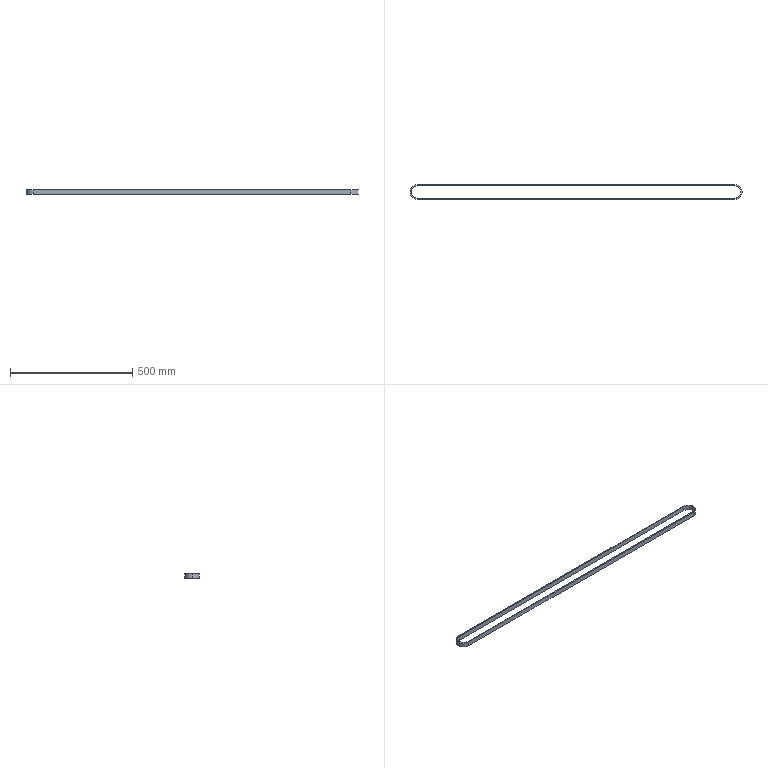Part | STEP file | Guide wheel mechanism revised.sldasm-Part-328 | 1 solid | 12 faces | box 1359 x 59 x 20 mm | volume 249410 mm3 | cylinder 6 | plane 6 | commonest cylinder face diameters 50 x3 59 x3
STEP:
#1=CARTESIAN_POINT('',(0.,25.,10.));
#2=VERTEX_POINT('',#1);
#3=CARTESIAN_POINT('',(-25.,0.,10.));
#4=VERTEX_POINT('',#3);
#5=CARTESIAN_POINT('',(0.,0.,10.));
#6=DIRECTION('',(0.,0.,1.));
#7=DIRECTION('',(1.,0.,0.));
#8=AXIS2_PLACEMENT_3D('',#5,#6,#7);
#9=CIRCLE('',#8,25.);
#10=EDGE_CURVE('',#2,#4,#9,.T.);
#11=ORIENTED_EDGE('',*,*,#10,.T.);
#12=CARTESIAN_POINT('',(-25.,0.,-10.));
#13=VERTEX_POINT('',#12);
#14=CARTESIAN_POINT('',(-25.,0.,10.));
#15=DIRECTION('',(0.,0.,-1.));
#16=VECTOR('',#15,1000.);
#17=LINE('',#14,#16);
#18=EDGE_CURVE('',#4,#13,#17,.T.);
#19=ORIENTED_EDGE('',*,*,#18,.T.);
#20=CARTESIAN_POINT('',(0.,25.,-10.));
#21=VERTEX_POINT('',#20);
#22=CARTESIAN_POINT('',(0.,0.,-10.));
#23=DIRECTION('',(0.,0.,1.));
#24=DIRECTION('',(1.,0.,0.));
#25=AXIS2_PLACEMENT_3D('',#22,#23,#24);
#26=CIRCLE('',#25,25.);
#27=EDGE_CURVE('',#21,#13,#26,.T.);
#28=ORIENTED_EDGE('',*,*,#27,.F.);
#29=CARTESIAN_POINT('',(0.,25.,10.));
#30=DIRECTION('',(0.,0.,-1.));
#31=VECTOR('',#30,1000.);
#32=LINE('',#29,#31);
#33=EDGE_CURVE('',#2,#21,#32,.T.);
#34=ORIENTED_EDGE('',*,*,#33,.F.);
#35=EDGE_LOOP('',(#11,#19,#28,#34));
#36=FACE_OUTER_BOUND('',#35,.T.);
#37=CARTESIAN_POINT('',(0.,0.,10.));
#38=DIRECTION('',(0.,0.,-1.));
#39=DIRECTION('',(-1.,0.,0.));
#40=AXIS2_PLACEMENT_3D('',#37,#38,#39);
#41=CYLINDRICAL_SURFACE('',#40,25.);
#42=ADVANCED_FACE('',(#36),#41,.F.);
#43=CARTESIAN_POINT('',(-29.5,0.,10.));
#44=VERTEX_POINT('',#43);
#45=CARTESIAN_POINT('',(0.,-29.5,10.));
#46=VERTEX_POINT('',#45);
#47=CARTESIAN_POINT('',(0.,0.,10.));
#48=DIRECTION('',(0.,0.,1.));
#49=DIRECTION('',(1.,0.,0.));
#50=AXIS2_PLACEMENT_3D('',#47,#48,#49);
#51=CIRCLE('',#50,29.5);
#52=EDGE_CURVE('',#44,#46,#51,.T.);
#53=ORIENTED_EDGE('',*,*,#52,.F.);
#54=CARTESIAN_POINT('',(-29.5,0.,-10.));
#55=VERTEX_POINT('',#54);
#56=CARTESIAN_POINT('',(-29.5,0.,10.));
#57=DIRECTION('',(0.,0.,-1.));
#58=VECTOR('',#57,1000.);
#59=LINE('',#56,#58);
#60=EDGE_CURVE('',#44,#55,#59,.T.);
#61=ORIENTED_EDGE('',*,*,#60,.T.);
#62=CARTESIAN_POINT('',(0.,-29.5,-10.));
#63=VERTEX_POINT('',#62);
#64=CARTESIAN_POINT('',(0.,0.,-10.));
#65=DIRECTION('',(0.,0.,1.));
#66=DIRECTION('',(1.,0.,0.));
#67=AXIS2_PLACEMENT_3D('',#64,#65,#66);
#68=CIRCLE('',#67,29.5);
#69=EDGE_CURVE('',#55,#63,#68,.T.);
#70=ORIENTED_EDGE('',*,*,#69,.T.);
#71=CARTESIAN_POINT('',(0.,-29.5,10.));
#72=DIRECTION('',(0.,0.,-1.));
#73=VECTOR('',#72,1000.);
#74=LINE('',#71,#73);
#75=EDGE_CURVE('',#46,#63,#74,.T.);
#76=ORIENTED_EDGE('',*,*,#75,.F.);
#77=EDGE_LOOP('',(#53,#61,#70,#76));
#78=FACE_OUTER_BOUND('',#77,.T.);
#79=CARTESIAN_POINT('',(0.,0.,10.));
#80=DIRECTION('',(0.,0.,-1.));
#81=DIRECTION('',(-1.,0.,0.));
#82=AXIS2_PLACEMENT_3D('',#79,#80,#81);
#83=CYLINDRICAL_SURFACE('',#82,29.5);
#84=ADVANCED_FACE('',(#78),#83,.T.);
#85=CARTESIAN_POINT('',(0.,29.5,10.));
#86=VERTEX_POINT('',#85);
#87=CARTESIAN_POINT('',(0.,0.,10.));
#88=DIRECTION('',(0.,0.,1.));
#89=DIRECTION('',(1.,0.,0.));
#90=AXIS2_PLACEMENT_3D('',#87,#88,#89);
#91=CIRCLE('',#90,29.5);
#92=EDGE_CURVE('',#86,#44,#91,.T.);
#93=ORIENTED_EDGE('',*,*,#92,.T.);
#94=ORIENTED_EDGE('',*,*,#52,.T.);
#95=CARTESIAN_POINT('',(1300.,-29.5,10.));
#96=VERTEX_POINT('',#95);
#97=CARTESIAN_POINT('',(0.,-29.5,10.));
#98=DIRECTION('',(1.,0.,0.));
#99=VECTOR('',#98,1000.);
#100=LINE('',#97,#99);
#101=EDGE_CURVE('',#46,#96,#100,.T.);
#102=ORIENTED_EDGE('',*,*,#101,.T.);
#103=CARTESIAN_POINT('',(1300.,29.5,10.));
#104=VERTEX_POINT('',#103);
#105=CARTESIAN_POINT('',(1300.,0.,10.));
#106=DIRECTION('',(0.,0.,1.));
#107=DIRECTION('',(1.,0.,0.));
#108=AXIS2_PLACEMENT_3D('',#105,#106,#107);
#109=CIRCLE('',#108,29.5);
#110=EDGE_CURVE('',#96,#104,#109,.T.);
#111=ORIENTED_EDGE('',*,*,#110,.T.);
#112=CARTESIAN_POINT('',(1300.,29.5,10.));
#113=DIRECTION('',(-1.,0.,0.));
#114=VECTOR('',#113,1000.);
#115=LINE('',#112,#114);
#116=EDGE_CURVE('',#104,#86,#115,.T.);
#117=ORIENTED_EDGE('',*,*,#116,.T.);
#118=EDGE_LOOP('',(#93,#94,#102,#111,#117));
#119=FACE_OUTER_BOUND('',#118,.T.);
#120=CARTESIAN_POINT('',(0.,-25.,10.));
#121=VERTEX_POINT('',#120);
#122=CARTESIAN_POINT('',(1300.,-25.,10.));
#123=VERTEX_POINT('',#122);
#124=CARTESIAN_POINT('',(0.,-25.,10.));
#125=DIRECTION('',(1.,0.,0.));
#126=VECTOR('',#125,1000.);
#127=LINE('',#124,#126);
#128=EDGE_CURVE('',#121,#123,#127,.T.);
#129=ORIENTED_EDGE('',*,*,#128,.F.);
#130=CARTESIAN_POINT('',(0.,0.,10.));
#131=DIRECTION('',(0.,0.,1.));
#132=DIRECTION('',(1.,0.,0.));
#133=AXIS2_PLACEMENT_3D('',#130,#131,#132);
#134=CIRCLE('',#133,25.);
#135=EDGE_CURVE('',#4,#121,#134,.T.);
#136=ORIENTED_EDGE('',*,*,#135,.F.);
#137=ORIENTED_EDGE('',*,*,#10,.F.);
#138=CARTESIAN_POINT('',(1300.,25.,10.));
#139=VERTEX_POINT('',#138);
#140=CARTESIAN_POINT('',(1300.,25.,10.));
#141=DIRECTION('',(-1.,0.,0.));
#142=VECTOR('',#141,1000.);
#143=LINE('',#140,#142);
#144=EDGE_CURVE('',#139,#2,#143,.T.);
#145=ORIENTED_EDGE('',*,*,#144,.F.);
#146=CARTESIAN_POINT('',(1300.,0.,10.));
#147=DIRECTION('',(0.,0.,1.));
#148=DIRECTION('',(1.,0.,0.));
#149=AXIS2_PLACEMENT_3D('',#146,#147,#148);
#150=CIRCLE('',#149,25.);
#151=EDGE_CURVE('',#123,#139,#150,.T.);
#152=ORIENTED_EDGE('',*,*,#151,.F.);
#153=EDGE_LOOP('',(#129,#136,#137,#145,#152));
#154=FACE_BOUND('',#153,.T.);
#155=CARTESIAN_POINT('',(0.,0.,10.));
#156=DIRECTION('',(0.,0.,1.));
#157=DIRECTION('',(1.,0.,0.));
#158=AXIS2_PLACEMENT_3D('',#155,#156,#157);
#159=PLANE('',#158);
#160=ADVANCED_FACE('',(#119,#154),#159,.T.);
#161=ORIENTED_EDGE('',*,*,#60,.F.);
#162=ORIENTED_EDGE('',*,*,#92,.F.);
#163=CARTESIAN_POINT('',(0.,29.5,-10.));
#164=VERTEX_POINT('',#163);
#165=CARTESIAN_POINT('',(0.,29.5,10.));
#166=DIRECTION('',(0.,0.,-1.));
#167=VECTOR('',#166,1000.);
#168=LINE('',#165,#167);
#169=EDGE_CURVE('',#86,#164,#168,.T.);
#170=ORIENTED_EDGE('',*,*,#169,.T.);
#171=CARTESIAN_POINT('',(0.,0.,-10.));
#172=DIRECTION('',(0.,0.,1.));
#173=DIRECTION('',(1.,0.,0.));
#174=AXIS2_PLACEMENT_3D('',#171,#172,#173);
#175=CIRCLE('',#174,29.5);
#176=EDGE_CURVE('',#164,#55,#175,.T.);
#177=ORIENTED_EDGE('',*,*,#176,.T.);
#178=EDGE_LOOP('',(#161,#162,#170,#177));
#179=FACE_OUTER_BOUND('',#178,.T.);
#180=CARTESIAN_POINT('',(0.,0.,10.));
#181=DIRECTION('',(0.,0.,-1.));
#182=DIRECTION('',(-1.,0.,0.));
#183=AXIS2_PLACEMENT_3D('',#180,#181,#182);
#184=CYLINDRICAL_SURFACE('',#183,29.5);
#185=ADVANCED_FACE('',(#179),#184,.T.);
#186=ORIENTED_EDGE('',*,*,#75,.T.);
#187=CARTESIAN_POINT('',(1300.,-29.5,-10.));
#188=VERTEX_POINT('',#187);
#189=CARTESIAN_POINT('',(0.,-29.5,-10.));
#190=DIRECTION('',(1.,0.,0.));
#191=VECTOR('',#190,1000.);
#192=LINE('',#189,#191);
#193=EDGE_CURVE('',#63,#188,#192,.T.);
#194=ORIENTED_EDGE('',*,*,#193,.T.);
#195=CARTESIAN_POINT('',(1300.,-29.5,10.));
#196=DIRECTION('',(0.,0.,-1.));
#197=VECTOR('',#196,1000.);
#198=LINE('',#195,#197);
#199=EDGE_CURVE('',#96,#188,#198,.T.);
#200=ORIENTED_EDGE('',*,*,#199,.F.);
#201=ORIENTED_EDGE('',*,*,#101,.F.);
#202=EDGE_LOOP('',(#186,#194,#200,#201));
#203=FACE_OUTER_BOUND('',#202,.T.);
#204=CARTESIAN_POINT('',(650.,-29.5,10.));
#205=DIRECTION('',(0.,1.,0.));
#206=DIRECTION('',(-1.,0.,0.));
#207=AXIS2_PLACEMENT_3D('',#204,#205,#206);
#208=PLANE('',#207);
#209=ADVANCED_FACE('',(#203),#208,.F.);
#210=ORIENTED_EDGE('',*,*,#199,.T.);
#211=CARTESIAN_POINT('',(1300.,29.5,-10.));
#212=VERTEX_POINT('',#211);
#213=CARTESIAN_POINT('',(1300.,0.,-10.));
#214=DIRECTION('',(0.,0.,1.));
#215=DIRECTION('',(1.,0.,0.));
#216=AXIS2_PLACEMENT_3D('',#213,#214,#215);
#217=CIRCLE('',#216,29.5);
#218=EDGE_CURVE('',#188,#212,#217,.T.);
#219=ORIENTED_EDGE('',*,*,#218,.T.);
#220=CARTESIAN_POINT('',(1300.,29.5,10.));
#221=DIRECTION('',(0.,0.,-1.));
#222=VECTOR('',#221,1000.);
#223=LINE('',#220,#222);
#224=EDGE_CURVE('',#104,#212,#223,.T.);
#225=ORIENTED_EDGE('',*,*,#224,.F.);
#226=ORIENTED_EDGE('',*,*,#110,.F.);
#227=EDGE_LOOP('',(#210,#219,#225,#226));
#228=FACE_OUTER_BOUND('',#227,.T.);
#229=CARTESIAN_POINT('',(1300.,0.,10.));
#230=DIRECTION('',(0.,0.,-1.));
#231=DIRECTION('',(-1.,0.,0.));
#232=AXIS2_PLACEMENT_3D('',#229,#230,#231);
#233=CYLINDRICAL_SURFACE('',#232,29.5);
#234=ADVANCED_FACE('',(#228),#233,.T.);
#235=ORIENTED_EDGE('',*,*,#224,.T.);
#236=CARTESIAN_POINT('',(1300.,29.5,-10.));
#237=DIRECTION('',(-1.,0.,0.));
#238=VECTOR('',#237,1000.);
#239=LINE('',#236,#238);
#240=EDGE_CURVE('',#212,#164,#239,.T.);
#241=ORIENTED_EDGE('',*,*,#240,.T.);
#242=ORIENTED_EDGE('',*,*,#169,.F.);
#243=ORIENTED_EDGE('',*,*,#116,.F.);
#244=EDGE_LOOP('',(#235,#241,#242,#243));
#245=FACE_OUTER_BOUND('',#244,.T.);
#246=CARTESIAN_POINT('',(1300.,29.5,10.));
#247=DIRECTION('',(0.,-1.,0.));
#248=DIRECTION('',(0.,0.,-1.));
#249=AXIS2_PLACEMENT_3D('',#246,#247,#248);
#250=PLANE('',#249);
#251=ADVANCED_FACE('',(#245),#250,.F.);
#252=ORIENTED_EDGE('',*,*,#18,.F.);
#253=ORIENTED_EDGE('',*,*,#135,.T.);
#254=CARTESIAN_POINT('',(0.,-25.,-10.));
#255=VERTEX_POINT('',#254);
#256=CARTESIAN_POINT('',(0.,-25.,10.));
#257=DIRECTION('',(0.,0.,-1.));
#258=VECTOR('',#257,1000.);
#259=LINE('',#256,#258);
#260=EDGE_CURVE('',#121,#255,#259,.T.);
#261=ORIENTED_EDGE('',*,*,#260,.T.);
#262=CARTESIAN_POINT('',(0.,0.,-10.));
#263=DIRECTION('',(0.,0.,1.));
#264=DIRECTION('',(1.,0.,0.));
#265=AXIS2_PLACEMENT_3D('',#262,#263,#264);
#266=CIRCLE('',#265,25.);
#267=EDGE_CURVE('',#13,#255,#266,.T.);
#268=ORIENTED_EDGE('',*,*,#267,.F.);
#269=EDGE_LOOP('',(#252,#253,#261,#268));
#270=FACE_OUTER_BOUND('',#269,.T.);
#271=CARTESIAN_POINT('',(0.,0.,10.));
#272=DIRECTION('',(0.,0.,-1.));
#273=DIRECTION('',(-1.,0.,0.));
#274=AXIS2_PLACEMENT_3D('',#271,#272,#273);
#275=CYLINDRICAL_SURFACE('',#274,25.);
#276=ADVANCED_FACE('',(#270),#275,.F.);
#277=CARTESIAN_POINT('',(1300.,-25.,-10.));
#278=VERTEX_POINT('',#277);
#279=CARTESIAN_POINT('',(1300.,-25.,10.));
#280=DIRECTION('',(0.,0.,-1.));
#281=VECTOR('',#280,1000.);
#282=LINE('',#279,#281);
#283=EDGE_CURVE('',#123,#278,#282,.T.);
#284=ORIENTED_EDGE('',*,*,#283,.T.);
#285=CARTESIAN_POINT('',(0.,-25.,-10.));
#286=DIRECTION('',(1.,0.,0.));
#287=VECTOR('',#286,1000.);
#288=LINE('',#285,#287);
#289=EDGE_CURVE('',#255,#278,#288,.T.);
#290=ORIENTED_EDGE('',*,*,#289,.F.);
#291=ORIENTED_EDGE('',*,*,#260,.F.);
#292=ORIENTED_EDGE('',*,*,#128,.T.);
#293=EDGE_LOOP('',(#284,#290,#291,#292));
#294=FACE_OUTER_BOUND('',#293,.T.);
#295=CARTESIAN_POINT('',(650.,-25.,10.));
#296=DIRECTION('',(0.,1.,0.));
#297=DIRECTION('',(-1.,0.,0.));
#298=AXIS2_PLACEMENT_3D('',#295,#296,#297);
#299=PLANE('',#298);
#300=ADVANCED_FACE('',(#294),#299,.T.);
#301=CARTESIAN_POINT('',(1300.,25.,-10.));
#302=VERTEX_POINT('',#301);
#303=CARTESIAN_POINT('',(1300.,25.,10.));
#304=DIRECTION('',(0.,0.,-1.));
#305=VECTOR('',#304,1000.);
#306=LINE('',#303,#305);
#307=EDGE_CURVE('',#139,#302,#306,.T.);
#308=ORIENTED_EDGE('',*,*,#307,.T.);
#309=CARTESIAN_POINT('',(1300.,0.,-10.));
#310=DIRECTION('',(0.,0.,1.));
#311=DIRECTION('',(1.,0.,0.));
#312=AXIS2_PLACEMENT_3D('',#309,#310,#311);
#313=CIRCLE('',#312,25.);
#314=EDGE_CURVE('',#278,#302,#313,.T.);
#315=ORIENTED_EDGE('',*,*,#314,.F.);
#316=ORIENTED_EDGE('',*,*,#283,.F.);
#317=ORIENTED_EDGE('',*,*,#151,.T.);
#318=EDGE_LOOP('',(#308,#315,#316,#317));
#319=FACE_OUTER_BOUND('',#318,.T.);
#320=CARTESIAN_POINT('',(1300.,0.,10.));
#321=DIRECTION('',(0.,0.,-1.));
#322=DIRECTION('',(-1.,0.,0.));
#323=AXIS2_PLACEMENT_3D('',#320,#321,#322);
#324=CYLINDRICAL_SURFACE('',#323,25.);
#325=ADVANCED_FACE('',(#319),#324,.F.);
#326=ORIENTED_EDGE('',*,*,#33,.T.);
#327=CARTESIAN_POINT('',(1300.,25.,-10.));
#328=DIRECTION('',(-1.,0.,0.));
#329=VECTOR('',#328,1000.);
#330=LINE('',#327,#329);
#331=EDGE_CURVE('',#302,#21,#330,.T.);
#332=ORIENTED_EDGE('',*,*,#331,.F.);
#333=ORIENTED_EDGE('',*,*,#307,.F.);
#334=ORIENTED_EDGE('',*,*,#144,.T.);
#335=EDGE_LOOP('',(#326,#332,#333,#334));
#336=FACE_OUTER_BOUND('',#335,.T.);
#337=CARTESIAN_POINT('',(1300.,25.,10.));
#338=DIRECTION('',(0.,-1.,0.));
#339=DIRECTION('',(0.,0.,-1.));
#340=AXIS2_PLACEMENT_3D('',#337,#338,#339);
#341=PLANE('',#340);
#342=ADVANCED_FACE('',(#336),#341,.T.);
#343=ORIENTED_EDGE('',*,*,#331,.T.);
#344=ORIENTED_EDGE('',*,*,#27,.T.);
#345=ORIENTED_EDGE('',*,*,#267,.T.);
#346=ORIENTED_EDGE('',*,*,#289,.T.);
#347=ORIENTED_EDGE('',*,*,#314,.T.);
#348=EDGE_LOOP('',(#343,#344,#345,#346,#347));
#349=FACE_BOUND('',#348,.T.);
#350=ORIENTED_EDGE('',*,*,#176,.F.);
#351=ORIENTED_EDGE('',*,*,#240,.F.);
#352=ORIENTED_EDGE('',*,*,#218,.F.);
#353=ORIENTED_EDGE('',*,*,#193,.F.);
#354=ORIENTED_EDGE('',*,*,#69,.F.);
#355=EDGE_LOOP('',(#350,#351,#352,#353,#354));
#356=FACE_OUTER_BOUND('',#355,.T.);
#357=CARTESIAN_POINT('',(0.,0.,-10.));
#358=DIRECTION('',(0.,0.,1.));
#359=DIRECTION('',(1.,0.,0.));
#360=AXIS2_PLACEMENT_3D('',#357,#358,#359);
#361=PLANE('',#360);
#362=ADVANCED_FACE('',(#349,#356),#361,.F.);
#363=CLOSED_SHELL('',(#42,#84,#160,#185,#209,#234,#251,#276,#300,#325,#342,#362));
#364=MANIFOLD_SOLID_BREP('',#363);
#365=CARTESIAN_POINT('',(0.,0.,0.));
#366=DIRECTION('',(0.,0.,1.));
#367=DIRECTION('',(1.,0.,0.));
#368=AXIS2_PLACEMENT_3D('',#365,#366,#367);
#369=(LENGTH_UNIT()NAMED_UNIT(*)SI_UNIT(.MILLI.,.METRE.));
#370=UNCERTAINTY_MEASURE_WITH_UNIT(LENGTH_MEASURE(0.00001),#369,'','');
#371=(NAMED_UNIT(*)PLANE_ANGLE_UNIT()SI_UNIT($,.RADIAN.));
#372=(NAMED_UNIT(*)SI_UNIT($,.STERADIAN.)SOLID_ANGLE_UNIT());
#373=(GEOMETRIC_REPRESENTATION_CONTEXT(3)GLOBAL_UNCERTAINTY_ASSIGNED_CONTEXT((#370))GLOBAL_UNIT_ASSIGNED_CONTEXT((#369,#371,#372))REPRESENTATION_CONTEXT('',''));
#374=ADVANCED_BREP_SHAPE_REPRESENTATION('',(#364,#368),#373);